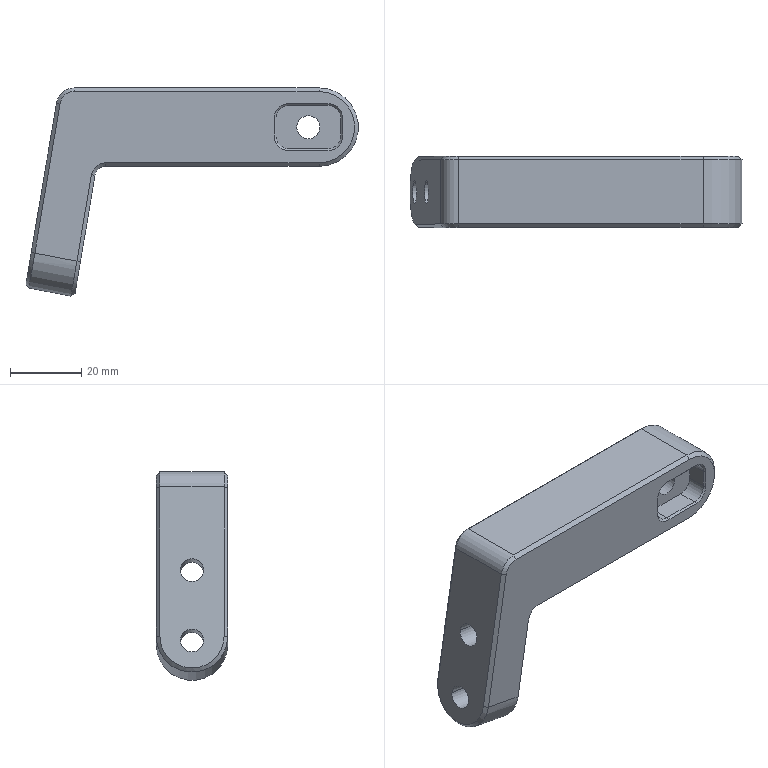Part | SolidWorks | features BaseBody 1 | 1 solid | 58 faces | box 93.242 x 20 x 58.451 mm | volume 41624 mm3 | plane 26 | cylinder 20 | cone 10 | spline 2 | commonest cylinder face diameters 6.5 x6 11 x6 7.2 x4 6 x1 10 x1 20 x1